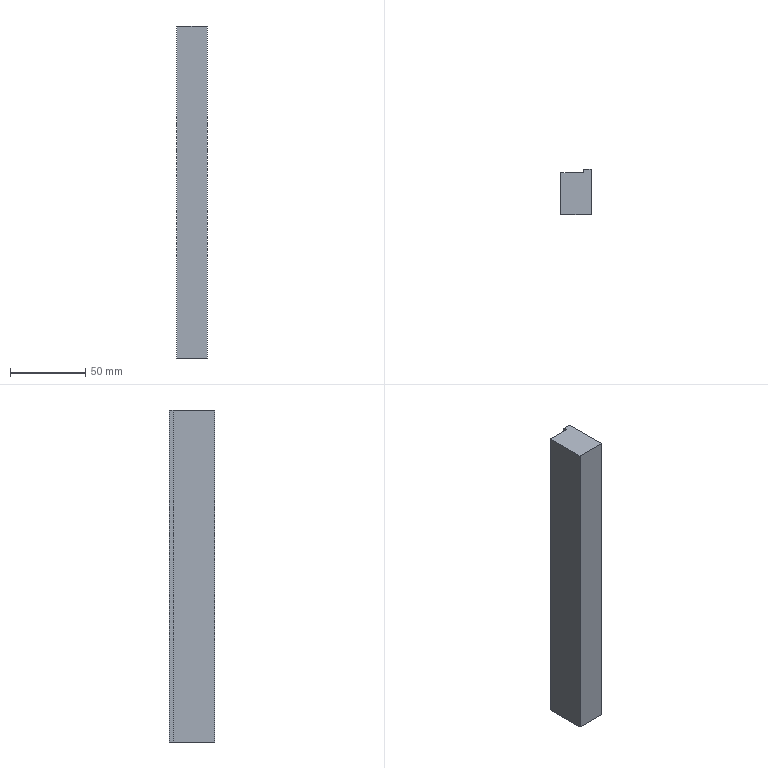Part | STEP file | 2012-06-08-02 | 1 solid | 8 faces | box 20 x 30 x 220 mm | volume 123750 mm3 | plane 8
STEP:
#1=CARTESIAN_POINT('',(0.,0.,0.));
#2=DIRECTION('',(0.,0.,1.));
#3=DIRECTION('',(1.,0.,0.));
#4=AXIS2_PLACEMENT_3D('',#1,#2,#3);
#5=CARTESIAN_POINT('',(0.,27.5,0.));
#6=VERTEX_POINT('',#5);
#7=CARTESIAN_POINT('',(0.,0.,0.));
#8=VERTEX_POINT('',#7);
#9=CARTESIAN_POINT('',(0.,0.,0.));
#10=DIRECTION('',(0.,-1.,0.));
#11=VECTOR('',#10,1.);
#12=LINE('',#9,#11);
#13=CARTESIAN_POINT('',(0.,0.,220.));
#14=DIRECTION('',(1.,0.,0.));
#15=DIRECTION('',(0.,0.,-1.));
#16=AXIS2_PLACEMENT_3D('',#13,#14,#15);
#17=PLANE('',#16);
#18=CARTESIAN_POINT('',(220.,0.));
#19=DIRECTION('',(0.,-1.));
#20=VECTOR('',#19,1.);
#21=LINE('',#18,#20);
#22=(GEOMETRIC_REPRESENTATION_CONTEXT(2)PARAMETRIC_REPRESENTATION_CONTEXT()REPRESENTATION_CONTEXT('',''));
#23=DEFINITIONAL_REPRESENTATION('',(#21),#22);
#24=PCURVE('',#17,#23);
#25=CARTESIAN_POINT('',(0.,27.5,0.));
#26=DIRECTION('',(0.,0.,1.));
#27=DIRECTION('',(1.,0.,0.));
#28=AXIS2_PLACEMENT_3D('',#25,#26,#27);
#29=PLANE('',#28);
#30=CARTESIAN_POINT('',(0.,-27.5));
#31=DIRECTION('',(0.,-1.));
#32=VECTOR('',#31,1.);
#33=LINE('',#30,#32);
#34=(GEOMETRIC_REPRESENTATION_CONTEXT(2)PARAMETRIC_REPRESENTATION_CONTEXT()REPRESENTATION_CONTEXT('',''));
#35=DEFINITIONAL_REPRESENTATION('',(#33),#34);
#36=PCURVE('',#29,#35);
#37=SURFACE_CURVE('',#12,(#24,#36),.PCURVE_S1.);
#38=EDGE_CURVE('',#6,#8,#37,.T.);
#39=ORIENTED_EDGE('',*,*,#38,.T.);
#40=CARTESIAN_POINT('',(0.,0.,220.));
#41=VERTEX_POINT('',#40);
#42=CARTESIAN_POINT('',(0.,0.,220.));
#43=DIRECTION('',(0.,0.,-1.));
#44=VECTOR('',#43,1.);
#45=LINE('',#42,#44);
#46=CARTESIAN_POINT('',(0.,0.));
#47=DIRECTION('',(1.,0.));
#48=VECTOR('',#47,1.);
#49=LINE('',#46,#48);
#50=(GEOMETRIC_REPRESENTATION_CONTEXT(2)PARAMETRIC_REPRESENTATION_CONTEXT()REPRESENTATION_CONTEXT('',''));
#51=DEFINITIONAL_REPRESENTATION('',(#49),#50);
#52=PCURVE('',#17,#51);
#53=CARTESIAN_POINT('',(0.,0.,220.));
#54=DIRECTION('',(0.,1.,0.));
#55=DIRECTION('',(0.,0.,1.));
#56=AXIS2_PLACEMENT_3D('',#53,#54,#55);
#57=PLANE('',#56);
#58=CARTESIAN_POINT('',(0.,0.));
#59=DIRECTION('',(-1.,0.));
#60=VECTOR('',#59,1.);
#61=LINE('',#58,#60);
#62=(GEOMETRIC_REPRESENTATION_CONTEXT(2)PARAMETRIC_REPRESENTATION_CONTEXT()REPRESENTATION_CONTEXT('',''));
#63=DEFINITIONAL_REPRESENTATION('',(#61),#62);
#64=PCURVE('',#57,#63);
#65=SURFACE_CURVE('',#45,(#52,#64),.PCURVE_S1.);
#66=EDGE_CURVE('',#41,#8,#65,.T.);
#67=ORIENTED_EDGE('',*,*,#66,.F.);
#68=CARTESIAN_POINT('',(0.,27.5,220.));
#69=VERTEX_POINT('',#68);
#70=CARTESIAN_POINT('',(0.,0.,220.));
#71=DIRECTION('',(0.,-1.,0.));
#72=VECTOR('',#71,1.);
#73=LINE('',#70,#72);
#74=CARTESIAN_POINT('',(0.,0.));
#75=DIRECTION('',(0.,-1.));
#76=VECTOR('',#75,1.);
#77=LINE('',#74,#76);
#78=(GEOMETRIC_REPRESENTATION_CONTEXT(2)PARAMETRIC_REPRESENTATION_CONTEXT()REPRESENTATION_CONTEXT('',''));
#79=DEFINITIONAL_REPRESENTATION('',(#77),#78);
#80=PCURVE('',#17,#79);
#81=CARTESIAN_POINT('',(0.,27.5,220.));
#82=DIRECTION('',(0.,0.,1.));
#83=DIRECTION('',(1.,0.,0.));
#84=AXIS2_PLACEMENT_3D('',#81,#82,#83);
#85=PLANE('',#84);
#86=CARTESIAN_POINT('',(0.,-27.5));
#87=DIRECTION('',(0.,-1.));
#88=VECTOR('',#87,1.);
#89=LINE('',#86,#88);
#90=(GEOMETRIC_REPRESENTATION_CONTEXT(2)PARAMETRIC_REPRESENTATION_CONTEXT()REPRESENTATION_CONTEXT('',''));
#91=DEFINITIONAL_REPRESENTATION('',(#89),#90);
#92=PCURVE('',#85,#91);
#93=SURFACE_CURVE('',#73,(#80,#92),.PCURVE_S1.);
#94=EDGE_CURVE('',#69,#41,#93,.T.);
#95=ORIENTED_EDGE('',*,*,#94,.F.);
#96=CARTESIAN_POINT('',(0.,27.5,220.));
#97=DIRECTION('',(0.,0.,-1.));
#98=VECTOR('',#97,1.);
#99=LINE('',#96,#98);
#100=CARTESIAN_POINT('',(0.,27.5));
#101=DIRECTION('',(1.,0.));
#102=VECTOR('',#101,1.);
#103=LINE('',#100,#102);
#104=(GEOMETRIC_REPRESENTATION_CONTEXT(2)PARAMETRIC_REPRESENTATION_CONTEXT()REPRESENTATION_CONTEXT('',''));
#105=DEFINITIONAL_REPRESENTATION('',(#103),#104);
#106=PCURVE('',#17,#105);
#107=CARTESIAN_POINT('',(15.,27.5,220.));
#108=DIRECTION('',(0.,-1.,0.));
#109=DIRECTION('',(1.,0.,0.));
#110=AXIS2_PLACEMENT_3D('',#107,#108,#109);
#111=PLANE('',#110);
#112=CARTESIAN_POINT('',(-15.,0.));
#113=DIRECTION('',(0.,-1.));
#114=VECTOR('',#113,1.);
#115=LINE('',#112,#114);
#116=(GEOMETRIC_REPRESENTATION_CONTEXT(2)PARAMETRIC_REPRESENTATION_CONTEXT()REPRESENTATION_CONTEXT('',''));
#117=DEFINITIONAL_REPRESENTATION('',(#115),#116);
#118=PCURVE('',#111,#117);
#119=SURFACE_CURVE('',#99,(#106,#118),.PCURVE_S1.);
#120=EDGE_CURVE('',#69,#6,#119,.T.);
#121=ORIENTED_EDGE('',*,*,#120,.T.);
#122=EDGE_LOOP('',(#39,#67,#95,#121));
#123=FACE_BOUND('',#122,.T.);
#124=ADVANCED_FACE('',(#123),#17,.F.);
#125=CARTESIAN_POINT('',(20.,0.,0.));
#126=VERTEX_POINT('',#125);
#127=CARTESIAN_POINT('',(0.,0.,0.));
#128=DIRECTION('',(1.,0.,0.));
#129=VECTOR('',#128,1.);
#130=LINE('',#127,#129);
#131=CARTESIAN_POINT('',(-220.,0.));
#132=DIRECTION('',(0.,1.));
#133=VECTOR('',#132,1.);
#134=LINE('',#131,#133);
#135=(GEOMETRIC_REPRESENTATION_CONTEXT(2)PARAMETRIC_REPRESENTATION_CONTEXT()REPRESENTATION_CONTEXT('',''));
#136=DEFINITIONAL_REPRESENTATION('',(#134),#135);
#137=PCURVE('',#57,#136);
#138=CARTESIAN_POINT('',(0.,-27.5));
#139=DIRECTION('',(1.,0.));
#140=VECTOR('',#139,1.);
#141=LINE('',#138,#140);
#142=(GEOMETRIC_REPRESENTATION_CONTEXT(2)PARAMETRIC_REPRESENTATION_CONTEXT()REPRESENTATION_CONTEXT('',''));
#143=DEFINITIONAL_REPRESENTATION('',(#141),#142);
#144=PCURVE('',#29,#143);
#145=SURFACE_CURVE('',#130,(#137,#144),.PCURVE_S1.);
#146=EDGE_CURVE('',#8,#126,#145,.T.);
#147=ORIENTED_EDGE('',*,*,#146,.T.);
#148=CARTESIAN_POINT('',(20.,0.,220.));
#149=VERTEX_POINT('',#148);
#150=CARTESIAN_POINT('',(20.,0.,220.));
#151=DIRECTION('',(0.,0.,-1.));
#152=VECTOR('',#151,1.);
#153=LINE('',#150,#152);
#154=CARTESIAN_POINT('',(0.,20.));
#155=DIRECTION('',(-1.,0.));
#156=VECTOR('',#155,1.);
#157=LINE('',#154,#156);
#158=(GEOMETRIC_REPRESENTATION_CONTEXT(2)PARAMETRIC_REPRESENTATION_CONTEXT()REPRESENTATION_CONTEXT('',''));
#159=DEFINITIONAL_REPRESENTATION('',(#157),#158);
#160=PCURVE('',#57,#159);
#161=CARTESIAN_POINT('',(20.,0.,220.));
#162=DIRECTION('',(-1.,0.,0.));
#163=DIRECTION('',(0.,-1.,0.));
#164=AXIS2_PLACEMENT_3D('',#161,#162,#163);
#165=PLANE('',#164);
#166=CARTESIAN_POINT('',(0.,0.));
#167=DIRECTION('',(0.,-1.));
#168=VECTOR('',#167,1.);
#169=LINE('',#166,#168);
#170=(GEOMETRIC_REPRESENTATION_CONTEXT(2)PARAMETRIC_REPRESENTATION_CONTEXT()REPRESENTATION_CONTEXT('',''));
#171=DEFINITIONAL_REPRESENTATION('',(#169),#170);
#172=PCURVE('',#165,#171);
#173=SURFACE_CURVE('',#153,(#160,#172),.PCURVE_S1.);
#174=EDGE_CURVE('',#149,#126,#173,.T.);
#175=ORIENTED_EDGE('',*,*,#174,.F.);
#176=CARTESIAN_POINT('',(0.,0.,220.));
#177=DIRECTION('',(1.,0.,0.));
#178=VECTOR('',#177,1.);
#179=LINE('',#176,#178);
#180=CARTESIAN_POINT('',(0.,0.));
#181=DIRECTION('',(0.,1.));
#182=VECTOR('',#181,1.);
#183=LINE('',#180,#182);
#184=(GEOMETRIC_REPRESENTATION_CONTEXT(2)PARAMETRIC_REPRESENTATION_CONTEXT()REPRESENTATION_CONTEXT('',''));
#185=DEFINITIONAL_REPRESENTATION('',(#183),#184);
#186=PCURVE('',#57,#185);
#187=CARTESIAN_POINT('',(0.,-27.5));
#188=DIRECTION('',(1.,0.));
#189=VECTOR('',#188,1.);
#190=LINE('',#187,#189);
#191=(GEOMETRIC_REPRESENTATION_CONTEXT(2)PARAMETRIC_REPRESENTATION_CONTEXT()REPRESENTATION_CONTEXT('',''));
#192=DEFINITIONAL_REPRESENTATION('',(#190),#191);
#193=PCURVE('',#85,#192);
#194=SURFACE_CURVE('',#179,(#186,#193),.PCURVE_S1.);
#195=EDGE_CURVE('',#41,#149,#194,.T.);
#196=ORIENTED_EDGE('',*,*,#195,.F.);
#197=ORIENTED_EDGE('',*,*,#66,.T.);
#198=EDGE_LOOP('',(#147,#175,#196,#197));
#199=FACE_BOUND('',#198,.T.);
#200=ADVANCED_FACE('',(#199),#57,.F.);
#201=CARTESIAN_POINT('',(20.,30.,0.));
#202=VERTEX_POINT('',#201);
#203=CARTESIAN_POINT('',(20.,0.,0.));
#204=DIRECTION('',(0.,1.,0.));
#205=VECTOR('',#204,1.);
#206=LINE('',#203,#205);
#207=CARTESIAN_POINT('',(0.,-220.));
#208=DIRECTION('',(-1.,0.));
#209=VECTOR('',#208,1.);
#210=LINE('',#207,#209);
#211=(GEOMETRIC_REPRESENTATION_CONTEXT(2)PARAMETRIC_REPRESENTATION_CONTEXT()REPRESENTATION_CONTEXT('',''));
#212=DEFINITIONAL_REPRESENTATION('',(#210),#211);
#213=PCURVE('',#165,#212);
#214=CARTESIAN_POINT('',(20.,-27.5));
#215=DIRECTION('',(0.,1.));
#216=VECTOR('',#215,1.);
#217=LINE('',#214,#216);
#218=(GEOMETRIC_REPRESENTATION_CONTEXT(2)PARAMETRIC_REPRESENTATION_CONTEXT()REPRESENTATION_CONTEXT('',''));
#219=DEFINITIONAL_REPRESENTATION('',(#217),#218);
#220=PCURVE('',#29,#219);
#221=SURFACE_CURVE('',#206,(#213,#220),.PCURVE_S1.);
#222=EDGE_CURVE('',#126,#202,#221,.T.);
#223=ORIENTED_EDGE('',*,*,#222,.T.);
#224=CARTESIAN_POINT('',(20.,30.,220.));
#225=VERTEX_POINT('',#224);
#226=CARTESIAN_POINT('',(20.,30.,220.));
#227=DIRECTION('',(0.,0.,-1.));
#228=VECTOR('',#227,1.);
#229=LINE('',#226,#228);
#230=CARTESIAN_POINT('',(-30.,0.));
#231=DIRECTION('',(0.,-1.));
#232=VECTOR('',#231,1.);
#233=LINE('',#230,#232);
#234=(GEOMETRIC_REPRESENTATION_CONTEXT(2)PARAMETRIC_REPRESENTATION_CONTEXT()REPRESENTATION_CONTEXT('',''));
#235=DEFINITIONAL_REPRESENTATION('',(#233),#234);
#236=PCURVE('',#165,#235);
#237=CARTESIAN_POINT('',(15.,30.,220.));
#238=DIRECTION('',(0.,-1.,0.));
#239=DIRECTION('',(0.,0.,-1.));
#240=AXIS2_PLACEMENT_3D('',#237,#238,#239);
#241=PLANE('',#240);
#242=CARTESIAN_POINT('',(0.,5.));
#243=DIRECTION('',(1.,0.));
#244=VECTOR('',#243,1.);
#245=LINE('',#242,#244);
#246=(GEOMETRIC_REPRESENTATION_CONTEXT(2)PARAMETRIC_REPRESENTATION_CONTEXT()REPRESENTATION_CONTEXT('',''));
#247=DEFINITIONAL_REPRESENTATION('',(#245),#246);
#248=PCURVE('',#241,#247);
#249=SURFACE_CURVE('',#229,(#236,#248),.PCURVE_S1.);
#250=EDGE_CURVE('',#225,#202,#249,.T.);
#251=ORIENTED_EDGE('',*,*,#250,.F.);
#252=CARTESIAN_POINT('',(20.,0.,220.));
#253=DIRECTION('',(0.,1.,0.));
#254=VECTOR('',#253,1.);
#255=LINE('',#252,#254);
#256=CARTESIAN_POINT('',(0.,0.));
#257=DIRECTION('',(-1.,0.));
#258=VECTOR('',#257,1.);
#259=LINE('',#256,#258);
#260=(GEOMETRIC_REPRESENTATION_CONTEXT(2)PARAMETRIC_REPRESENTATION_CONTEXT()REPRESENTATION_CONTEXT('',''));
#261=DEFINITIONAL_REPRESENTATION('',(#259),#260);
#262=PCURVE('',#165,#261);
#263=CARTESIAN_POINT('',(20.,-27.5));
#264=DIRECTION('',(0.,1.));
#265=VECTOR('',#264,1.);
#266=LINE('',#263,#265);
#267=(GEOMETRIC_REPRESENTATION_CONTEXT(2)PARAMETRIC_REPRESENTATION_CONTEXT()REPRESENTATION_CONTEXT('',''));
#268=DEFINITIONAL_REPRESENTATION('',(#266),#267);
#269=PCURVE('',#85,#268);
#270=SURFACE_CURVE('',#255,(#262,#269),.PCURVE_S1.);
#271=EDGE_CURVE('',#149,#225,#270,.T.);
#272=ORIENTED_EDGE('',*,*,#271,.F.);
#273=ORIENTED_EDGE('',*,*,#174,.T.);
#274=EDGE_LOOP('',(#223,#251,#272,#273));
#275=FACE_BOUND('',#274,.T.);
#276=ADVANCED_FACE('',(#275),#165,.F.);
#277=CARTESIAN_POINT('',(15.,30.,0.));
#278=VERTEX_POINT('',#277);
#279=CARTESIAN_POINT('',(15.,30.,0.));
#280=DIRECTION('',(-1.,0.,0.));
#281=VECTOR('',#280,1.);
#282=LINE('',#279,#281);
#283=CARTESIAN_POINT('',(220.,0.));
#284=DIRECTION('',(0.,-1.));
#285=VECTOR('',#284,1.);
#286=LINE('',#283,#285);
#287=(GEOMETRIC_REPRESENTATION_CONTEXT(2)PARAMETRIC_REPRESENTATION_CONTEXT()REPRESENTATION_CONTEXT('',''));
#288=DEFINITIONAL_REPRESENTATION('',(#286),#287);
#289=PCURVE('',#241,#288);
#290=CARTESIAN_POINT('',(15.,2.5));
#291=DIRECTION('',(-1.,0.));
#292=VECTOR('',#291,1.);
#293=LINE('',#290,#292);
#294=(GEOMETRIC_REPRESENTATION_CONTEXT(2)PARAMETRIC_REPRESENTATION_CONTEXT()REPRESENTATION_CONTEXT('',''));
#295=DEFINITIONAL_REPRESENTATION('',(#293),#294);
#296=PCURVE('',#29,#295);
#297=SURFACE_CURVE('',#282,(#289,#296),.PCURVE_S1.);
#298=EDGE_CURVE('',#202,#278,#297,.T.);
#299=ORIENTED_EDGE('',*,*,#298,.T.);
#300=CARTESIAN_POINT('',(15.,30.,220.));
#301=VERTEX_POINT('',#300);
#302=CARTESIAN_POINT('',(15.,30.,220.));
#303=DIRECTION('',(0.,0.,-1.));
#304=VECTOR('',#303,1.);
#305=LINE('',#302,#304);
#306=CARTESIAN_POINT('',(0.,0.));
#307=DIRECTION('',(1.,0.));
#308=VECTOR('',#307,1.);
#309=LINE('',#306,#308);
#310=(GEOMETRIC_REPRESENTATION_CONTEXT(2)PARAMETRIC_REPRESENTATION_CONTEXT()REPRESENTATION_CONTEXT('',''));
#311=DEFINITIONAL_REPRESENTATION('',(#309),#310);
#312=PCURVE('',#241,#311);
#313=CARTESIAN_POINT('',(15.,30.,220.));
#314=DIRECTION('',(1.,0.,0.));
#315=DIRECTION('',(0.,0.,-1.));
#316=AXIS2_PLACEMENT_3D('',#313,#314,#315);
#317=PLANE('',#316);
#318=CARTESIAN_POINT('',(0.,0.));
#319=DIRECTION('',(1.,0.));
#320=VECTOR('',#319,1.);
#321=LINE('',#318,#320);
#322=(GEOMETRIC_REPRESENTATION_CONTEXT(2)PARAMETRIC_REPRESENTATION_CONTEXT()REPRESENTATION_CONTEXT('',''));
#323=DEFINITIONAL_REPRESENTATION('',(#321),#322);
#324=PCURVE('',#317,#323);
#325=SURFACE_CURVE('',#305,(#312,#324),.PCURVE_S1.);
#326=EDGE_CURVE('',#301,#278,#325,.T.);
#327=ORIENTED_EDGE('',*,*,#326,.F.);
#328=CARTESIAN_POINT('',(15.,30.,220.));
#329=DIRECTION('',(-1.,0.,0.));
#330=VECTOR('',#329,1.);
#331=LINE('',#328,#330);
#332=CARTESIAN_POINT('',(0.,0.));
#333=DIRECTION('',(0.,-1.));
#334=VECTOR('',#333,1.);
#335=LINE('',#332,#334);
#336=(GEOMETRIC_REPRESENTATION_CONTEXT(2)PARAMETRIC_REPRESENTATION_CONTEXT()REPRESENTATION_CONTEXT('',''));
#337=DEFINITIONAL_REPRESENTATION('',(#335),#336);
#338=PCURVE('',#241,#337);
#339=CARTESIAN_POINT('',(15.,2.5));
#340=DIRECTION('',(-1.,0.));
#341=VECTOR('',#340,1.);
#342=LINE('',#339,#341);
#343=(GEOMETRIC_REPRESENTATION_CONTEXT(2)PARAMETRIC_REPRESENTATION_CONTEXT()REPRESENTATION_CONTEXT('',''));
#344=DEFINITIONAL_REPRESENTATION('',(#342),#343);
#345=PCURVE('',#85,#344);
#346=SURFACE_CURVE('',#331,(#338,#345),.PCURVE_S1.);
#347=EDGE_CURVE('',#225,#301,#346,.T.);
#348=ORIENTED_EDGE('',*,*,#347,.F.);
#349=ORIENTED_EDGE('',*,*,#250,.T.);
#350=EDGE_LOOP('',(#299,#327,#348,#349));
#351=FACE_BOUND('',#350,.T.);
#352=ADVANCED_FACE('',(#351),#241,.F.);
#353=CARTESIAN_POINT('',(15.,27.5,0.));
#354=VERTEX_POINT('',#353);
#355=CARTESIAN_POINT('',(15.,30.,0.));
#356=DIRECTION('',(0.,-1.,0.));
#357=VECTOR('',#356,1.);
#358=LINE('',#355,#357);
#359=CARTESIAN_POINT('',(220.,0.));
#360=DIRECTION('',(0.,-1.));
#361=VECTOR('',#360,1.);
#362=LINE('',#359,#361);
#363=(GEOMETRIC_REPRESENTATION_CONTEXT(2)PARAMETRIC_REPRESENTATION_CONTEXT()REPRESENTATION_CONTEXT('',''));
#364=DEFINITIONAL_REPRESENTATION('',(#362),#363);
#365=PCURVE('',#317,#364);
#366=CARTESIAN_POINT('',(15.,2.5));
#367=DIRECTION('',(0.,-1.));
#368=VECTOR('',#367,1.);
#369=LINE('',#366,#368);
#370=(GEOMETRIC_REPRESENTATION_CONTEXT(2)PARAMETRIC_REPRESENTATION_CONTEXT()REPRESENTATION_CONTEXT('',''));
#371=DEFINITIONAL_REPRESENTATION('',(#369),#370);
#372=PCURVE('',#29,#371);
#373=SURFACE_CURVE('',#358,(#365,#372),.PCURVE_S1.);
#374=EDGE_CURVE('',#278,#354,#373,.T.);
#375=ORIENTED_EDGE('',*,*,#374,.T.);
#376=CARTESIAN_POINT('',(15.,27.5,220.));
#377=VERTEX_POINT('',#376);
#378=CARTESIAN_POINT('',(15.,27.5,220.));
#379=DIRECTION('',(0.,0.,-1.));
#380=VECTOR('',#379,1.);
#381=LINE('',#378,#380);
#382=CARTESIAN_POINT('',(0.,-2.5));
#383=DIRECTION('',(1.,0.));
#384=VECTOR('',#383,1.);
#385=LINE('',#382,#384);
#386=(GEOMETRIC_REPRESENTATION_CONTEXT(2)PARAMETRIC_REPRESENTATION_CONTEXT()REPRESENTATION_CONTEXT('',''));
#387=DEFINITIONAL_REPRESENTATION('',(#385),#386);
#388=PCURVE('',#317,#387);
#389=CARTESIAN_POINT('',(0.,0.));
#390=DIRECTION('',(0.,-1.));
#391=VECTOR('',#390,1.);
#392=LINE('',#389,#391);
#393=(GEOMETRIC_REPRESENTATION_CONTEXT(2)PARAMETRIC_REPRESENTATION_CONTEXT()REPRESENTATION_CONTEXT('',''));
#394=DEFINITIONAL_REPRESENTATION('',(#392),#393);
#395=PCURVE('',#111,#394);
#396=SURFACE_CURVE('',#381,(#388,#395),.PCURVE_S1.);
#397=EDGE_CURVE('',#377,#354,#396,.T.);
#398=ORIENTED_EDGE('',*,*,#397,.F.);
#399=CARTESIAN_POINT('',(15.,30.,220.));
#400=DIRECTION('',(0.,-1.,0.));
#401=VECTOR('',#400,1.);
#402=LINE('',#399,#401);
#403=CARTESIAN_POINT('',(0.,0.));
#404=DIRECTION('',(0.,-1.));
#405=VECTOR('',#404,1.);
#406=LINE('',#403,#405);
#407=(GEOMETRIC_REPRESENTATION_CONTEXT(2)PARAMETRIC_REPRESENTATION_CONTEXT()REPRESENTATION_CONTEXT('',''));
#408=DEFINITIONAL_REPRESENTATION('',(#406),#407);
#409=PCURVE('',#317,#408);
#410=CARTESIAN_POINT('',(15.,2.5));
#411=DIRECTION('',(0.,-1.));
#412=VECTOR('',#411,1.);
#413=LINE('',#410,#412);
#414=(GEOMETRIC_REPRESENTATION_CONTEXT(2)PARAMETRIC_REPRESENTATION_CONTEXT()REPRESENTATION_CONTEXT('',''));
#415=DEFINITIONAL_REPRESENTATION('',(#413),#414);
#416=PCURVE('',#85,#415);
#417=SURFACE_CURVE('',#402,(#409,#416),.PCURVE_S1.);
#418=EDGE_CURVE('',#301,#377,#417,.T.);
#419=ORIENTED_EDGE('',*,*,#418,.F.);
#420=ORIENTED_EDGE('',*,*,#326,.T.);
#421=EDGE_LOOP('',(#375,#398,#419,#420));
#422=FACE_BOUND('',#421,.T.);
#423=ADVANCED_FACE('',(#422),#317,.F.);
#424=CARTESIAN_POINT('',(15.,27.5,0.));
#425=DIRECTION('',(-1.,0.,0.));
#426=VECTOR('',#425,1.);
#427=LINE('',#424,#426);
#428=CARTESIAN_POINT('',(0.,-220.));
#429=DIRECTION('',(-1.,0.));
#430=VECTOR('',#429,1.);
#431=LINE('',#428,#430);
#432=(GEOMETRIC_REPRESENTATION_CONTEXT(2)PARAMETRIC_REPRESENTATION_CONTEXT()REPRESENTATION_CONTEXT('',''));
#433=DEFINITIONAL_REPRESENTATION('',(#431),#432);
#434=PCURVE('',#111,#433);
#435=CARTESIAN_POINT('',(15.,0.));
#436=DIRECTION('',(-1.,0.));
#437=VECTOR('',#436,1.);
#438=LINE('',#435,#437);
#439=(GEOMETRIC_REPRESENTATION_CONTEXT(2)PARAMETRIC_REPRESENTATION_CONTEXT()REPRESENTATION_CONTEXT('',''));
#440=DEFINITIONAL_REPRESENTATION('',(#438),#439);
#441=PCURVE('',#29,#440);
#442=SURFACE_CURVE('',#427,(#434,#441),.PCURVE_S1.);
#443=EDGE_CURVE('',#354,#6,#442,.T.);
#444=ORIENTED_EDGE('',*,*,#443,.T.);
#445=ORIENTED_EDGE('',*,*,#120,.F.);
#446=CARTESIAN_POINT('',(15.,27.5,220.));
#447=DIRECTION('',(-1.,0.,0.));
#448=VECTOR('',#447,1.);
#449=LINE('',#446,#448);
#450=CARTESIAN_POINT('',(0.,0.));
#451=DIRECTION('',(-1.,0.));
#452=VECTOR('',#451,1.);
#453=LINE('',#450,#452);
#454=(GEOMETRIC_REPRESENTATION_CONTEXT(2)PARAMETRIC_REPRESENTATION_CONTEXT()REPRESENTATION_CONTEXT('',''));
#455=DEFINITIONAL_REPRESENTATION('',(#453),#454);
#456=PCURVE('',#111,#455);
#457=CARTESIAN_POINT('',(15.,0.));
#458=DIRECTION('',(-1.,0.));
#459=VECTOR('',#458,1.);
#460=LINE('',#457,#459);
#461=(GEOMETRIC_REPRESENTATION_CONTEXT(2)PARAMETRIC_REPRESENTATION_CONTEXT()REPRESENTATION_CONTEXT('',''));
#462=DEFINITIONAL_REPRESENTATION('',(#460),#461);
#463=PCURVE('',#85,#462);
#464=SURFACE_CURVE('',#449,(#456,#463),.PCURVE_S1.);
#465=EDGE_CURVE('',#377,#69,#464,.T.);
#466=ORIENTED_EDGE('',*,*,#465,.F.);
#467=ORIENTED_EDGE('',*,*,#397,.T.);
#468=EDGE_LOOP('',(#444,#445,#466,#467));
#469=FACE_BOUND('',#468,.T.);
#470=ADVANCED_FACE('',(#469),#111,.F.);
#471=ORIENTED_EDGE('',*,*,#94,.T.);
#472=ORIENTED_EDGE('',*,*,#195,.T.);
#473=ORIENTED_EDGE('',*,*,#271,.T.);
#474=ORIENTED_EDGE('',*,*,#347,.T.);
#475=ORIENTED_EDGE('',*,*,#418,.T.);
#476=ORIENTED_EDGE('',*,*,#465,.T.);
#477=EDGE_LOOP('',(#471,#472,#473,#474,#475,#476));
#478=FACE_BOUND('',#477,.T.);
#479=ADVANCED_FACE('',(#478),#85,.T.);
#480=ORIENTED_EDGE('',*,*,#38,.F.);
#481=ORIENTED_EDGE('',*,*,#443,.F.);
#482=ORIENTED_EDGE('',*,*,#374,.F.);
#483=ORIENTED_EDGE('',*,*,#298,.F.);
#484=ORIENTED_EDGE('',*,*,#222,.F.);
#485=ORIENTED_EDGE('',*,*,#146,.F.);
#486=EDGE_LOOP('',(#480,#481,#482,#483,#484,#485));
#487=FACE_BOUND('',#486,.T.);
#488=ADVANCED_FACE('',(#487),#29,.F.);
#489=CLOSED_SHELL('',(#124,#200,#276,#352,#423,#470,#479,#488));
#490=MANIFOLD_SOLID_BREP('',#489);
#491=(LENGTH_UNIT()NAMED_UNIT(*)SI_UNIT(.MILLI.,.METRE.));
#492=UNCERTAINTY_MEASURE_WITH_UNIT(LENGTH_MEASURE(0.0000001),#491,'','');
#493=(NAMED_UNIT(*)PLANE_ANGLE_UNIT()SI_UNIT($,.RADIAN.));
#494=(NAMED_UNIT(*)SI_UNIT($,.STERADIAN.)SOLID_ANGLE_UNIT());
#495=(GEOMETRIC_REPRESENTATION_CONTEXT(3)GLOBAL_UNCERTAINTY_ASSIGNED_CONTEXT((#492))GLOBAL_UNIT_ASSIGNED_CONTEXT((#491,#493,#494))REPRESENTATION_CONTEXT('',''));
#496=ADVANCED_BREP_SHAPE_REPRESENTATION('',(#4,#490),#495);